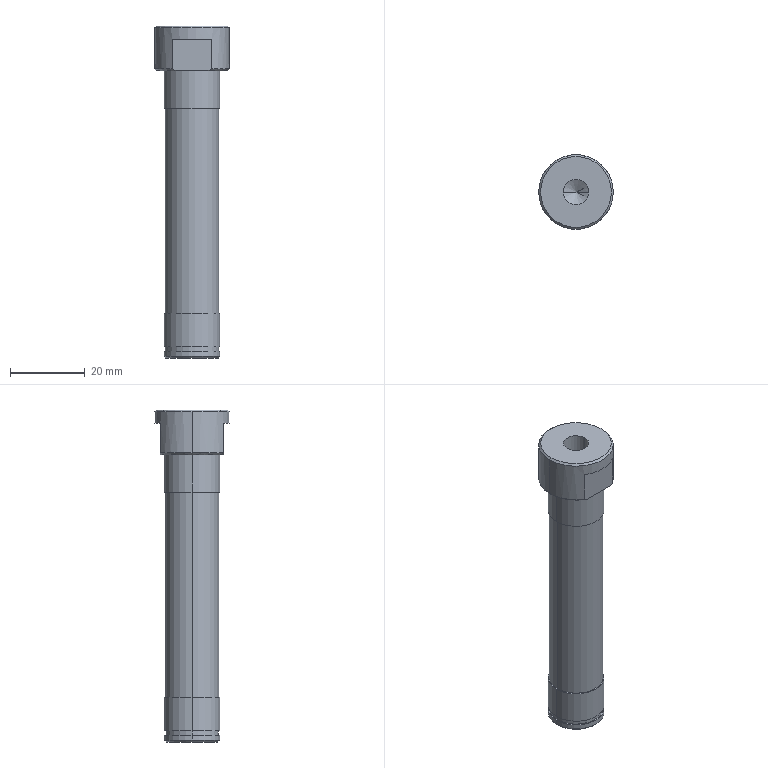Part | STEP file | 10000020461swp000-1 | 1 solid | 34 faces | box 20 x 20 x 89 mm | volume 15653 mm3 | cylinder 14 | plane 11 | cone 9 | commonest cylinder face diameters 15 x6 6.8 x2 14.3 x2 14.4 x2 20 x2
STEP:
#1=CARTESIAN_POINT('',(9.5,0.,0.));
#2=VERTEX_POINT('',#1);
#3=CARTESIAN_POINT('',(-9.5,0.,0.));
#4=VERTEX_POINT('',#3);
#5=CARTESIAN_POINT('',(0.,0.,0.));
#6=DIRECTION('',(0.,0.,1.));
#7=DIRECTION('',(1.,0.,0.));
#8=AXIS2_PLACEMENT_3D('',#5,#6,#7);
#9=CIRCLE('',#8,9.5);
#10=EDGE_CURVE('',#2,#4,#9,.T.);
#11=ORIENTED_EDGE('',*,*,#10,.F.);
#12=CARTESIAN_POINT('',(10.,0.,-0.5));
#13=VERTEX_POINT('',#12);
#14=CARTESIAN_POINT('',(9.5,0.,0.));
#15=DIRECTION('',(0.7071,0.,-0.7071));
#16=VECTOR('',#15,1000.);
#17=LINE('',#14,#16);
#18=EDGE_CURVE('',#2,#13,#17,.T.);
#19=ORIENTED_EDGE('',*,*,#18,.T.);
#20=CARTESIAN_POINT('',(-10.,0.,-0.5));
#21=VERTEX_POINT('',#20);
#22=CARTESIAN_POINT('',(0.,0.,-0.5));
#23=DIRECTION('',(0.,0.,-1.));
#24=DIRECTION('',(1.,0.,0.));
#25=AXIS2_PLACEMENT_3D('',#22,#23,#24);
#26=CIRCLE('',#25,10.);
#27=EDGE_CURVE('',#21,#13,#26,.T.);
#28=ORIENTED_EDGE('',*,*,#27,.F.);
#29=CARTESIAN_POINT('',(-9.5,0.,0.));
#30=DIRECTION('',(-0.7071,0.,-0.7071));
#31=VECTOR('',#30,1000.);
#32=LINE('',#29,#31);
#33=EDGE_CURVE('',#4,#21,#32,.T.);
#34=ORIENTED_EDGE('',*,*,#33,.F.);
#35=EDGE_LOOP('',(#11,#19,#28,#34));
#36=FACE_OUTER_BOUND('',#35,.T.);
#37=CARTESIAN_POINT('',(0.,0.,0.));
#38=DIRECTION('',(0.,0.,-1.));
#39=DIRECTION('',(-1.,0.,0.));
#40=AXIS2_PLACEMENT_3D('',#37,#38,#39);
#41=CONICAL_SURFACE('',#40,9.5,0.7854);
#42=ADVANCED_FACE('',(#36),#41,.T.);
#43=CARTESIAN_POINT('',(-7.,0.,-89.));
#44=VERTEX_POINT('',#43);
#45=CARTESIAN_POINT('',(7.,0.,-89.));
#46=VERTEX_POINT('',#45);
#47=CARTESIAN_POINT('',(0.,0.,-89.));
#48=DIRECTION('',(0.,0.,-1.));
#49=DIRECTION('',(-1.,0.,0.));
#50=AXIS2_PLACEMENT_3D('',#47,#48,#49);
#51=CIRCLE('',#50,7.);
#52=EDGE_CURVE('',#44,#46,#51,.T.);
#53=ORIENTED_EDGE('',*,*,#52,.F.);
#54=CARTESIAN_POINT('',(-7.5,0.,-88.5));
#55=VERTEX_POINT('',#54);
#56=CARTESIAN_POINT('',(-7.,0.,-89.));
#57=DIRECTION('',(-0.7071,0.,0.7071));
#58=VECTOR('',#57,1000.);
#59=LINE('',#56,#58);
#60=EDGE_CURVE('',#44,#55,#59,.T.);
#61=ORIENTED_EDGE('',*,*,#60,.T.);
#62=CARTESIAN_POINT('',(7.5,0.,-88.5));
#63=VERTEX_POINT('',#62);
#64=CARTESIAN_POINT('',(0.,0.,-88.5));
#65=DIRECTION('',(0.,0.,1.));
#66=DIRECTION('',(-1.,0.,0.));
#67=AXIS2_PLACEMENT_3D('',#64,#65,#66);
#68=CIRCLE('',#67,7.5);
#69=EDGE_CURVE('',#63,#55,#68,.T.);
#70=ORIENTED_EDGE('',*,*,#69,.F.);
#71=CARTESIAN_POINT('',(7.,0.,-89.));
#72=DIRECTION('',(0.7071,0.,0.7071));
#73=VECTOR('',#72,1000.);
#74=LINE('',#71,#73);
#75=EDGE_CURVE('',#46,#63,#74,.T.);
#76=ORIENTED_EDGE('',*,*,#75,.F.);
#77=EDGE_LOOP('',(#53,#61,#70,#76));
#78=FACE_OUTER_BOUND('',#77,.T.);
#79=CARTESIAN_POINT('',(0.,0.,-89.));
#80=DIRECTION('',(0.,0.,1.));
#81=DIRECTION('',(1.,0.,0.));
#82=AXIS2_PLACEMENT_3D('',#79,#80,#81);
#83=CONICAL_SURFACE('',#82,7.,0.7854);
#84=ADVANCED_FACE('',(#78),#83,.T.);
#85=CARTESIAN_POINT('',(9.5,0.,-12.));
#86=VERTEX_POINT('',#85);
#87=CARTESIAN_POINT('',(4.243,-8.5,-12.));
#88=VERTEX_POINT('',#87);
#89=CARTESIAN_POINT('',(0.,0.,-12.));
#90=DIRECTION('',(0.,0.,-1.));
#91=DIRECTION('',(1.,0.,0.));
#92=AXIS2_PLACEMENT_3D('',#89,#90,#91);
#93=CIRCLE('',#92,9.5);
#94=EDGE_CURVE('',#86,#88,#93,.T.);
#95=ORIENTED_EDGE('',*,*,#94,.F.);
#96=CARTESIAN_POINT('',(10.,0.,-11.5));
#97=VERTEX_POINT('',#96);
#98=CARTESIAN_POINT('',(10.,0.,-11.5));
#99=DIRECTION('',(0.7071,0.,0.7071));
#100=VECTOR('',#99,1000.);
#101=LINE('',#98,#100);
#102=EDGE_CURVE('',#86,#97,#101,.T.);
#103=ORIENTED_EDGE('',*,*,#102,.T.);
#104=CARTESIAN_POINT('',(5.268,-8.5,-11.5));
#105=VERTEX_POINT('',#104);
#106=CARTESIAN_POINT('',(0.,0.,-11.5));
#107=DIRECTION('',(0.,0.,1.));
#108=DIRECTION('',(1.,0.,0.));
#109=AXIS2_PLACEMENT_3D('',#106,#107,#108);
#110=CIRCLE('',#109,10.);
#111=EDGE_CURVE('',#105,#97,#110,.T.);
#112=ORIENTED_EDGE('',*,*,#111,.F.);
#113=CARTESIAN_POINT('',(4.243,-8.5,-12.));
#114=CARTESIAN_POINT('',(4.59,-8.5,-11.845));
#115=CARTESIAN_POINT('',(4.931,-8.5,-11.677));
#116=CARTESIAN_POINT('',(5.268,-8.5,-11.5));
#117=B_SPLINE_CURVE_WITH_KNOTS('',3,(#113,#114,#115,#116),.UNSPECIFIED.,.F.,.F.,(4,4),(0.,0.001141),.UNSPECIFIED.);
#118=EDGE_CURVE('',#88,#105,#117,.T.);
#119=ORIENTED_EDGE('',*,*,#118,.F.);
#120=EDGE_LOOP('',(#95,#103,#112,#119));
#121=FACE_OUTER_BOUND('',#120,.T.);
#122=CARTESIAN_POINT('',(0.,0.,-11.5));
#123=DIRECTION('',(0.,0.,1.));
#124=DIRECTION('',(1.,0.,0.));
#125=AXIS2_PLACEMENT_3D('',#122,#123,#124);
#126=CONICAL_SURFACE('',#125,10.,0.7854);
#127=ADVANCED_FACE('',(#121),#126,.T.);
#128=CARTESIAN_POINT('',(-3.4,0.,-19.75));
#129=VERTEX_POINT('',#128);
#130=CARTESIAN_POINT('',(3.4,0.,-19.75));
#131=VERTEX_POINT('',#130);
#132=CARTESIAN_POINT('',(0.,0.,-19.75));
#133=DIRECTION('',(0.,0.,1.));
#134=DIRECTION('',(1.,0.,0.));
#135=AXIS2_PLACEMENT_3D('',#132,#133,#134);
#136=CIRCLE('',#135,3.4);
#137=EDGE_CURVE('',#129,#131,#136,.T.);
#138=ORIENTED_EDGE('',*,*,#137,.F.);
#139=CARTESIAN_POINT('',(-3.4,0.,0.));
#140=VERTEX_POINT('',#139);
#141=CARTESIAN_POINT('',(-3.4,0.,0.));
#142=DIRECTION('',(0.,0.,1.));
#143=VECTOR('',#142,1000.);
#144=LINE('',#141,#143);
#145=EDGE_CURVE('',#129,#140,#144,.T.);
#146=ORIENTED_EDGE('',*,*,#145,.T.);
#147=CARTESIAN_POINT('',(3.4,0.,0.));
#148=VERTEX_POINT('',#147);
#149=CARTESIAN_POINT('',(0.,0.,0.));
#150=DIRECTION('',(0.,0.,1.));
#151=DIRECTION('',(1.,0.,0.));
#152=AXIS2_PLACEMENT_3D('',#149,#150,#151);
#153=CIRCLE('',#152,3.4);
#154=EDGE_CURVE('',#140,#148,#153,.T.);
#155=ORIENTED_EDGE('',*,*,#154,.T.);
#156=CARTESIAN_POINT('',(3.4,0.,0.));
#157=DIRECTION('',(0.,0.,1.));
#158=VECTOR('',#157,1000.);
#159=LINE('',#156,#158);
#160=EDGE_CURVE('',#131,#148,#159,.T.);
#161=ORIENTED_EDGE('',*,*,#160,.F.);
#162=EDGE_LOOP('',(#138,#146,#155,#161));
#163=FACE_OUTER_BOUND('',#162,.T.);
#164=CARTESIAN_POINT('',(0.,0.,0.));
#165=DIRECTION('',(0.,0.,1.));
#166=DIRECTION('',(1.,0.,0.));
#167=AXIS2_PLACEMENT_3D('',#164,#165,#166);
#168=CYLINDRICAL_SURFACE('',#167,3.4);
#169=ADVANCED_FACE('',(#163),#168,.F.);
#170=CARTESIAN_POINT('',(0.,0.,-21.793));
#171=VERTEX_POINT('',#170);
#172=CARTESIAN_POINT('',(3.4,0.,-19.75));
#173=DIRECTION('',(0.8572,0.,0.515));
#174=VECTOR('',#173,1000.);
#175=LINE('',#172,#174);
#176=EDGE_CURVE('',#171,#131,#175,.T.);
#177=ORIENTED_EDGE('',*,*,#176,.F.);
#178=CARTESIAN_POINT('',(-3.4,0.,-19.75));
#179=DIRECTION('',(-0.8572,0.,0.515));
#180=VECTOR('',#179,1000.);
#181=LINE('',#178,#180);
#182=EDGE_CURVE('',#171,#129,#181,.T.);
#183=ORIENTED_EDGE('',*,*,#182,.T.);
#184=ORIENTED_EDGE('',*,*,#137,.T.);
#185=EDGE_LOOP('',(#177,#183,#184));
#186=FACE_OUTER_BOUND('',#185,.T.);
#187=CARTESIAN_POINT('',(0.,0.,-19.75));
#188=DIRECTION('',(0.,0.,1.));
#189=DIRECTION('',(1.,0.,0.));
#190=AXIS2_PLACEMENT_3D('',#187,#188,#189);
#191=CONICAL_SURFACE('',#190,3.4,1.03);
#192=ADVANCED_FACE('',(#186),#191,.F.);
#193=ORIENTED_EDGE('',*,*,#69,.T.);
#194=CARTESIAN_POINT('',(-7.5,0.,-87.2));
#195=VERTEX_POINT('',#194);
#196=CARTESIAN_POINT('',(-7.5,0.,-89.));
#197=DIRECTION('',(0.,0.,1.));
#198=VECTOR('',#197,1000.);
#199=LINE('',#196,#198);
#200=EDGE_CURVE('',#55,#195,#199,.T.);
#201=ORIENTED_EDGE('',*,*,#200,.T.);
#202=CARTESIAN_POINT('',(7.5,0.,-87.2));
#203=VERTEX_POINT('',#202);
#204=CARTESIAN_POINT('',(0.,0.,-87.2));
#205=DIRECTION('',(0.,0.,-1.));
#206=DIRECTION('',(-1.,0.,0.));
#207=AXIS2_PLACEMENT_3D('',#204,#205,#206);
#208=CIRCLE('',#207,7.5);
#209=EDGE_CURVE('',#195,#203,#208,.T.);
#210=ORIENTED_EDGE('',*,*,#209,.T.);
#211=CARTESIAN_POINT('',(7.5,0.,-89.));
#212=DIRECTION('',(0.,0.,1.));
#213=VECTOR('',#212,1000.);
#214=LINE('',#211,#213);
#215=EDGE_CURVE('',#63,#203,#214,.T.);
#216=ORIENTED_EDGE('',*,*,#215,.F.);
#217=EDGE_LOOP('',(#193,#201,#210,#216));
#218=FACE_OUTER_BOUND('',#217,.T.);
#219=CARTESIAN_POINT('',(0.,0.,-89.));
#220=DIRECTION('',(0.,0.,1.));
#221=DIRECTION('',(1.,0.,0.));
#222=AXIS2_PLACEMENT_3D('',#219,#220,#221);
#223=CYLINDRICAL_SURFACE('',#222,7.5);
#224=ADVANCED_FACE('',(#218),#223,.T.);
#225=CARTESIAN_POINT('',(-7.15,0.,-86.));
#226=VERTEX_POINT('',#225);
#227=CARTESIAN_POINT('',(7.15,0.,-86.));
#228=VERTEX_POINT('',#227);
#229=CARTESIAN_POINT('',(0.,0.,-86.));
#230=DIRECTION('',(0.,0.,-1.));
#231=DIRECTION('',(-1.,0.,0.));
#232=AXIS2_PLACEMENT_3D('',#229,#230,#231);
#233=CIRCLE('',#232,7.15);
#234=EDGE_CURVE('',#226,#228,#233,.T.);
#235=ORIENTED_EDGE('',*,*,#234,.T.);
#236=CARTESIAN_POINT('',(7.15,0.,-87.2));
#237=VERTEX_POINT('',#236);
#238=CARTESIAN_POINT('',(7.15,0.,-89.));
#239=DIRECTION('',(0.,0.,-1.));
#240=VECTOR('',#239,1000.);
#241=LINE('',#238,#240);
#242=EDGE_CURVE('',#228,#237,#241,.T.);
#243=ORIENTED_EDGE('',*,*,#242,.T.);
#244=CARTESIAN_POINT('',(-7.15,0.,-87.2));
#245=VERTEX_POINT('',#244);
#246=CARTESIAN_POINT('',(0.,0.,-87.2));
#247=DIRECTION('',(0.,0.,-1.));
#248=DIRECTION('',(-1.,0.,0.));
#249=AXIS2_PLACEMENT_3D('',#246,#247,#248);
#250=CIRCLE('',#249,7.15);
#251=EDGE_CURVE('',#245,#237,#250,.T.);
#252=ORIENTED_EDGE('',*,*,#251,.F.);
#253=CARTESIAN_POINT('',(-7.15,0.,-89.));
#254=DIRECTION('',(0.,0.,-1.));
#255=VECTOR('',#254,1000.);
#256=LINE('',#253,#255);
#257=EDGE_CURVE('',#226,#245,#256,.T.);
#258=ORIENTED_EDGE('',*,*,#257,.F.);
#259=EDGE_LOOP('',(#235,#243,#252,#258));
#260=FACE_OUTER_BOUND('',#259,.T.);
#261=CARTESIAN_POINT('',(0.,0.,-89.));
#262=DIRECTION('',(0.,0.,-1.));
#263=DIRECTION('',(-1.,0.,0.));
#264=AXIS2_PLACEMENT_3D('',#261,#262,#263);
#265=CYLINDRICAL_SURFACE('',#264,7.15);
#266=ADVANCED_FACE('',(#260),#265,.T.);
#267=CARTESIAN_POINT('',(-7.2,0.,-77.));
#268=VERTEX_POINT('',#267);
#269=CARTESIAN_POINT('',(7.2,0.,-77.));
#270=VERTEX_POINT('',#269);
#271=CARTESIAN_POINT('',(0.,0.,-77.));
#272=DIRECTION('',(0.,0.,-1.));
#273=DIRECTION('',(-1.,0.,0.));
#274=AXIS2_PLACEMENT_3D('',#271,#272,#273);
#275=CIRCLE('',#274,7.2);
#276=EDGE_CURVE('',#268,#270,#275,.T.);
#277=ORIENTED_EDGE('',*,*,#276,.F.);
#278=CARTESIAN_POINT('',(-7.2,0.,-22.));
#279=VERTEX_POINT('',#278);
#280=CARTESIAN_POINT('',(-7.2,0.,-77.));
#281=DIRECTION('',(0.,0.,1.));
#282=VECTOR('',#281,1000.);
#283=LINE('',#280,#282);
#284=EDGE_CURVE('',#268,#279,#283,.T.);
#285=ORIENTED_EDGE('',*,*,#284,.T.);
#286=CARTESIAN_POINT('',(7.2,0.,-22.));
#287=VERTEX_POINT('',#286);
#288=CARTESIAN_POINT('',(0.,0.,-22.));
#289=DIRECTION('',(0.,0.,-1.));
#290=DIRECTION('',(-1.,0.,0.));
#291=AXIS2_PLACEMENT_3D('',#288,#289,#290);
#292=CIRCLE('',#291,7.2);
#293=EDGE_CURVE('',#279,#287,#292,.T.);
#294=ORIENTED_EDGE('',*,*,#293,.T.);
#295=CARTESIAN_POINT('',(7.2,0.,-77.));
#296=DIRECTION('',(0.,0.,1.));
#297=VECTOR('',#296,1000.);
#298=LINE('',#295,#297);
#299=EDGE_CURVE('',#270,#287,#298,.T.);
#300=ORIENTED_EDGE('',*,*,#299,.F.);
#301=EDGE_LOOP('',(#277,#285,#294,#300));
#302=FACE_OUTER_BOUND('',#301,.T.);
#303=CARTESIAN_POINT('',(0.,0.,-77.));
#304=DIRECTION('',(0.,0.,1.));
#305=DIRECTION('',(1.,0.,0.));
#306=AXIS2_PLACEMENT_3D('',#303,#304,#305);
#307=CYLINDRICAL_SURFACE('',#306,7.2);
#308=ADVANCED_FACE('',(#302),#307,.T.);
#309=CARTESIAN_POINT('',(-7.5,0.,-22.));
#310=VERTEX_POINT('',#309);
#311=CARTESIAN_POINT('',(7.5,0.,-22.));
#312=VERTEX_POINT('',#311);
#313=CARTESIAN_POINT('',(0.,0.,-22.));
#314=DIRECTION('',(0.,0.,-1.));
#315=DIRECTION('',(-1.,0.,0.));
#316=AXIS2_PLACEMENT_3D('',#313,#314,#315);
#317=CIRCLE('',#316,7.5);
#318=EDGE_CURVE('',#310,#312,#317,.T.);
#319=ORIENTED_EDGE('',*,*,#318,.F.);
#320=CARTESIAN_POINT('',(-7.5,0.,-12.));
#321=VERTEX_POINT('',#320);
#322=CARTESIAN_POINT('',(-7.5,0.,-22.));
#323=DIRECTION('',(0.,0.,1.));
#324=VECTOR('',#323,1000.);
#325=LINE('',#322,#324);
#326=EDGE_CURVE('',#310,#321,#325,.T.);
#327=ORIENTED_EDGE('',*,*,#326,.T.);
#328=CARTESIAN_POINT('',(7.5,0.,-12.));
#329=VERTEX_POINT('',#328);
#330=CARTESIAN_POINT('',(0.,0.,-12.));
#331=DIRECTION('',(0.,0.,-1.));
#332=DIRECTION('',(1.,0.,0.));
#333=AXIS2_PLACEMENT_3D('',#330,#331,#332);
#334=CIRCLE('',#333,7.5);
#335=EDGE_CURVE('',#321,#329,#334,.T.);
#336=ORIENTED_EDGE('',*,*,#335,.T.);
#337=CARTESIAN_POINT('',(7.5,0.,-22.));
#338=DIRECTION('',(0.,0.,1.));
#339=VECTOR('',#338,1000.);
#340=LINE('',#337,#339);
#341=EDGE_CURVE('',#312,#329,#340,.T.);
#342=ORIENTED_EDGE('',*,*,#341,.F.);
#343=EDGE_LOOP('',(#319,#327,#336,#342));
#344=FACE_OUTER_BOUND('',#343,.T.);
#345=CARTESIAN_POINT('',(0.,0.,-22.));
#346=DIRECTION('',(0.,0.,1.));
#347=DIRECTION('',(1.,0.,0.));
#348=AXIS2_PLACEMENT_3D('',#345,#346,#347);
#349=CYLINDRICAL_SURFACE('',#348,7.5);
#350=ADVANCED_FACE('',(#344),#349,.T.);
#351=CARTESIAN_POINT('',(-7.5,0.,-86.));
#352=VERTEX_POINT('',#351);
#353=CARTESIAN_POINT('',(7.5,0.,-86.));
#354=VERTEX_POINT('',#353);
#355=CARTESIAN_POINT('',(0.,0.,-86.));
#356=DIRECTION('',(0.,0.,-1.));
#357=DIRECTION('',(-1.,0.,0.));
#358=AXIS2_PLACEMENT_3D('',#355,#356,#357);
#359=CIRCLE('',#358,7.5);
#360=EDGE_CURVE('',#352,#354,#359,.T.);
#361=ORIENTED_EDGE('',*,*,#360,.F.);
#362=CARTESIAN_POINT('',(-7.5,0.,-77.));
#363=VERTEX_POINT('',#362);
#364=CARTESIAN_POINT('',(-7.5,0.,-89.));
#365=DIRECTION('',(0.,0.,1.));
#366=VECTOR('',#365,1000.);
#367=LINE('',#364,#366);
#368=EDGE_CURVE('',#352,#363,#367,.T.);
#369=ORIENTED_EDGE('',*,*,#368,.T.);
#370=CARTESIAN_POINT('',(7.5,0.,-77.));
#371=VERTEX_POINT('',#370);
#372=CARTESIAN_POINT('',(0.,0.,-77.));
#373=DIRECTION('',(0.,0.,-1.));
#374=DIRECTION('',(-1.,0.,0.));
#375=AXIS2_PLACEMENT_3D('',#372,#373,#374);
#376=CIRCLE('',#375,7.5);
#377=EDGE_CURVE('',#363,#371,#376,.T.);
#378=ORIENTED_EDGE('',*,*,#377,.T.);
#379=CARTESIAN_POINT('',(7.5,0.,-89.));
#380=DIRECTION('',(0.,0.,1.));
#381=VECTOR('',#380,1000.);
#382=LINE('',#379,#381);
#383=EDGE_CURVE('',#354,#371,#382,.T.);
#384=ORIENTED_EDGE('',*,*,#383,.F.);
#385=EDGE_LOOP('',(#361,#369,#378,#384));
#386=FACE_OUTER_BOUND('',#385,.T.);
#387=CARTESIAN_POINT('',(0.,0.,-89.));
#388=DIRECTION('',(0.,0.,1.));
#389=DIRECTION('',(1.,0.,0.));
#390=AXIS2_PLACEMENT_3D('',#387,#388,#389);
#391=CYLINDRICAL_SURFACE('',#390,7.5);
#392=ADVANCED_FACE('',(#386),#391,.T.);
#393=CARTESIAN_POINT('',(-5.268,8.5,-11.5));
#394=VERTEX_POINT('',#393);
#395=CARTESIAN_POINT('',(-10.,0.,-11.5));
#396=VERTEX_POINT('',#395);
#397=CARTESIAN_POINT('',(0.,0.,-11.5));
#398=DIRECTION('',(0.,0.,1.));
#399=DIRECTION('',(1.,0.,0.));
#400=AXIS2_PLACEMENT_3D('',#397,#398,#399);
#401=CIRCLE('',#400,10.);
#402=EDGE_CURVE('',#394,#396,#401,.T.);
#403=ORIENTED_EDGE('',*,*,#402,.T.);
#404=CARTESIAN_POINT('',(-10.,0.,-12.));
#405=DIRECTION('',(0.,0.,1.));
#406=VECTOR('',#405,1000.);
#407=LINE('',#404,#406);
#408=EDGE_CURVE('',#396,#21,#407,.T.);
#409=ORIENTED_EDGE('',*,*,#408,.T.);
#410=ORIENTED_EDGE('',*,*,#27,.T.);
#411=CARTESIAN_POINT('',(10.,0.,-12.));
#412=DIRECTION('',(0.,0.,1.));
#413=VECTOR('',#412,1000.);
#414=LINE('',#411,#413);
#415=EDGE_CURVE('',#97,#13,#414,.T.);
#416=ORIENTED_EDGE('',*,*,#415,.F.);
#417=CARTESIAN_POINT('',(5.268,8.5,-11.5));
#418=VERTEX_POINT('',#417);
#419=CARTESIAN_POINT('',(0.,0.,-11.5));
#420=DIRECTION('',(0.,0.,1.));
#421=DIRECTION('',(1.,0.,0.));
#422=AXIS2_PLACEMENT_3D('',#419,#420,#421);
#423=CIRCLE('',#422,10.);
#424=EDGE_CURVE('',#97,#418,#423,.T.);
#425=ORIENTED_EDGE('',*,*,#424,.T.);
#426=CARTESIAN_POINT('',(5.268,8.5,-3.5));
#427=VERTEX_POINT('',#426);
#428=CARTESIAN_POINT('',(5.268,8.5,-12.));
#429=DIRECTION('',(0.,0.,1.));
#430=VECTOR('',#429,1000.);
#431=LINE('',#428,#430);
#432=EDGE_CURVE('',#418,#427,#431,.T.);
#433=ORIENTED_EDGE('',*,*,#432,.T.);
#434=CARTESIAN_POINT('',(-5.268,8.5,-3.5));
#435=VERTEX_POINT('',#434);
#436=CARTESIAN_POINT('',(0.,0.,-3.5));
#437=DIRECTION('',(0.,0.,1.));
#438=DIRECTION('',(-1.,0.,0.));
#439=AXIS2_PLACEMENT_3D('',#436,#437,#438);
#440=CIRCLE('',#439,10.);
#441=EDGE_CURVE('',#427,#435,#440,.T.);
#442=ORIENTED_EDGE('',*,*,#441,.T.);
#443=CARTESIAN_POINT('',(-5.268,8.5,-12.));
#444=DIRECTION('',(0.,0.,-1.));
#445=VECTOR('',#444,1000.);
#446=LINE('',#443,#445);
#447=EDGE_CURVE('',#435,#394,#446,.T.);
#448=ORIENTED_EDGE('',*,*,#447,.T.);
#449=EDGE_LOOP('',(#403,#409,#410,#416,#425,#433,#442,#448));
#450=FACE_OUTER_BOUND('',#449,.T.);
#451=CARTESIAN_POINT('',(0.,0.,-12.));
#452=DIRECTION('',(0.,0.,1.));
#453=DIRECTION('',(1.,0.,0.));
#454=AXIS2_PLACEMENT_3D('',#451,#452,#453);
#455=CYLINDRICAL_SURFACE('',#454,10.);
#456=ADVANCED_FACE('',(#450),#455,.T.);
#457=ORIENTED_EDGE('',*,*,#408,.F.);
#458=CARTESIAN_POINT('',(-5.268,-8.5,-11.5));
#459=VERTEX_POINT('',#458);
#460=CARTESIAN_POINT('',(0.,0.,-11.5));
#461=DIRECTION('',(0.,0.,1.));
#462=DIRECTION('',(1.,0.,0.));
#463=AXIS2_PLACEMENT_3D('',#460,#461,#462);
#464=CIRCLE('',#463,10.);
#465=EDGE_CURVE('',#396,#459,#464,.T.);
#466=ORIENTED_EDGE('',*,*,#465,.T.);
#467=CARTESIAN_POINT('',(-5.268,-8.5,-3.5));
#468=VERTEX_POINT('',#467);
#469=CARTESIAN_POINT('',(-5.268,-8.5,-12.));
#470=DIRECTION('',(0.,0.,1.));
#471=VECTOR('',#470,1000.);
#472=LINE('',#469,#471);
#473=EDGE_CURVE('',#459,#468,#472,.T.);
#474=ORIENTED_EDGE('',*,*,#473,.T.);
#475=CARTESIAN_POINT('',(5.268,-8.5,-3.5));
#476=VERTEX_POINT('',#475);
#477=CARTESIAN_POINT('',(0.,0.,-3.5));
#478=DIRECTION('',(0.,0.,-1.));
#479=DIRECTION('',(1.,0.,0.));
#480=AXIS2_PLACEMENT_3D('',#477,#478,#479);
#481=CIRCLE('',#480,10.);
#482=EDGE_CURVE('',#476,#468,#481,.T.);
#483=ORIENTED_EDGE('',*,*,#482,.F.);
#484=CARTESIAN_POINT('',(5.268,-8.5,-12.));
#485=DIRECTION('',(0.,0.,-1.));
#486=VECTOR('',#485,1000.);
#487=LINE('',#484,#486);
#488=EDGE_CURVE('',#476,#105,#487,.T.);
#489=ORIENTED_EDGE('',*,*,#488,.T.);
#490=ORIENTED_EDGE('',*,*,#111,.T.);
#491=ORIENTED_EDGE('',*,*,#415,.T.);
#492=CARTESIAN_POINT('',(0.,0.,-0.5));
#493=DIRECTION('',(0.,0.,-1.));
#494=DIRECTION('',(1.,0.,0.));
#495=AXIS2_PLACEMENT_3D('',#492,#493,#494);
#496=CIRCLE('',#495,10.);
#497=EDGE_CURVE('',#13,#21,#496,.T.);
#498=ORIENTED_EDGE('',*,*,#497,.T.);
#499=EDGE_LOOP('',(#457,#466,#474,#483,#489,#490,#491,#498));
#500=FACE_OUTER_BOUND('',#499,.T.);
#501=CARTESIAN_POINT('',(0.,0.,-12.));
#502=DIRECTION('',(0.,0.,1.));
#503=DIRECTION('',(1.,0.,0.));
#504=AXIS2_PLACEMENT_3D('',#501,#502,#503);
#505=CYLINDRICAL_SURFACE('',#504,10.);
#506=ADVANCED_FACE('',(#500),#505,.T.);
#507=CARTESIAN_POINT('',(0.,0.,-12.));
#508=DIRECTION('',(0.,0.,-1.));
#509=DIRECTION('',(1.,0.,0.));
#510=AXIS2_PLACEMENT_3D('',#507,#508,#509);
#511=CIRCLE('',#510,7.5);
#512=EDGE_CURVE('',#329,#321,#511,.T.);
#513=ORIENTED_EDGE('',*,*,#512,.F.);
#514=ORIENTED_EDGE('',*,*,#335,.F.);
#515=EDGE_LOOP('',(#513,#514));
#516=FACE_BOUND('',#515,.T.);
#517=CARTESIAN_POINT('',(4.243,8.5,-12.));
#518=VERTEX_POINT('',#517);
#519=CARTESIAN_POINT('',(-4.243,8.5,-12.));
#520=VERTEX_POINT('',#519);
#521=CARTESIAN_POINT('',(0.,8.5,-12.));
#522=DIRECTION('',(-1.,0.,0.));
#523=VECTOR('',#522,1000.);
#524=LINE('',#521,#523);
#525=EDGE_CURVE('',#518,#520,#524,.T.);
#526=ORIENTED_EDGE('',*,*,#525,.F.);
#527=CARTESIAN_POINT('',(0.,0.,-12.));
#528=DIRECTION('',(0.,0.,-1.));
#529=DIRECTION('',(1.,0.,0.));
#530=AXIS2_PLACEMENT_3D('',#527,#528,#529);
#531=CIRCLE('',#530,9.5);
#532=EDGE_CURVE('',#518,#86,#531,.T.);
#533=ORIENTED_EDGE('',*,*,#532,.T.);
#534=ORIENTED_EDGE('',*,*,#94,.T.);
#535=CARTESIAN_POINT('',(-4.243,-8.5,-12.));
#536=VERTEX_POINT('',#535);
#537=CARTESIAN_POINT('',(0.,-8.5,-12.));
#538=DIRECTION('',(1.,0.,0.));
#539=VECTOR('',#538,1000.);
#540=LINE('',#537,#539);
#541=EDGE_CURVE('',#536,#88,#540,.T.);
#542=ORIENTED_EDGE('',*,*,#541,.F.);
#543=CARTESIAN_POINT('',(0.,0.,-12.));
#544=DIRECTION('',(0.,0.,-1.));
#545=DIRECTION('',(1.,0.,0.));
#546=AXIS2_PLACEMENT_3D('',#543,#544,#545);
#547=CIRCLE('',#546,9.5);
#548=EDGE_CURVE('',#536,#520,#547,.T.);
#549=ORIENTED_EDGE('',*,*,#548,.T.);
#550=EDGE_LOOP('',(#526,#533,#534,#542,#549));
#551=FACE_OUTER_BOUND('',#550,.T.);
#552=CARTESIAN_POINT('',(0.,0.,-12.));
#553=DIRECTION('',(0.,0.,1.));
#554=DIRECTION('',(1.,0.,0.));
#555=AXIS2_PLACEMENT_3D('',#552,#553,#554);
#556=PLANE('',#555);
#557=ADVANCED_FACE('',(#516,#551),#556,.F.);
#558=ORIENTED_EDGE('',*,*,#368,.F.);
#559=CARTESIAN_POINT('',(0.,0.,-86.));
#560=DIRECTION('',(0.,0.,-1.));
#561=DIRECTION('',(-1.,0.,0.));
#562=AXIS2_PLACEMENT_3D('',#559,#560,#561);
#563=CIRCLE('',#562,7.5);
#564=EDGE_CURVE('',#354,#352,#563,.T.);
#565=ORIENTED_EDGE('',*,*,#564,.F.);
#566=ORIENTED_EDGE('',*,*,#383,.T.);
#567=CARTESIAN_POINT('',(0.,0.,-77.));
#568=DIRECTION('',(0.,0.,-1.));
#569=DIRECTION('',(-1.,0.,0.));
#570=AXIS2_PLACEMENT_3D('',#567,#568,#569);
#571=CIRCLE('',#570,7.5);
#572=EDGE_CURVE('',#371,#363,#571,.T.);
#573=ORIENTED_EDGE('',*,*,#572,.T.);
#574=EDGE_LOOP('',(#558,#565,#566,#573));
#575=FACE_OUTER_BOUND('',#574,.T.);
#576=CARTESIAN_POINT('',(0.,0.,-89.));
#577=DIRECTION('',(0.,0.,1.));
#578=DIRECTION('',(1.,0.,0.));
#579=AXIS2_PLACEMENT_3D('',#576,#577,#578);
#580=CYLINDRICAL_SURFACE('',#579,7.5);
#581=ADVANCED_FACE('',(#575),#580,.T.);
#582=CARTESIAN_POINT('',(0.,0.,0.));
#583=DIRECTION('',(0.,0.,1.));
#584=DIRECTION('',(1.,0.,0.));
#585=AXIS2_PLACEMENT_3D('',#582,#583,#584);
#586=CIRCLE('',#585,9.5);
#587=EDGE_CURVE('',#4,#2,#586,.T.);
#588=ORIENTED_EDGE('',*,*,#587,.T.);
#589=ORIENTED_EDGE('',*,*,#10,.T.);
#590=EDGE_LOOP('',(#588,#589));
#591=FACE_OUTER_BOUND('',#590,.T.);
#592=CARTESIAN_POINT('',(0.,0.,0.));
#593=DIRECTION('',(0.,0.,1.));
#594=DIRECTION('',(1.,0.,0.));
#595=AXIS2_PLACEMENT_3D('',#592,#593,#594);
#596=CIRCLE('',#595,3.4);
#597=EDGE_CURVE('',#148,#140,#596,.T.);
#598=ORIENTED_EDGE('',*,*,#597,.F.);
#599=ORIENTED_EDGE('',*,*,#154,.F.);
#600=EDGE_LOOP('',(#598,#599));
#601=FACE_BOUND('',#600,.T.);
#602=CARTESIAN_POINT('',(0.,0.,0.));
#603=DIRECTION('',(0.,0.,1.));
#604=DIRECTION('',(1.,0.,0.));
#605=AXIS2_PLACEMENT_3D('',#602,#603,#604);
#606=PLANE('',#605);
#607=ADVANCED_FACE('',(#591,#601),#606,.T.);
#608=ORIENTED_EDGE('',*,*,#326,.F.);
#609=CARTESIAN_POINT('',(0.,0.,-22.));
#610=DIRECTION('',(0.,0.,-1.));
#611=DIRECTION('',(-1.,0.,0.));
#612=AXIS2_PLACEMENT_3D('',#609,#610,#611);
#613=CIRCLE('',#612,7.5);
#614=EDGE_CURVE('',#312,#310,#613,.T.);
#615=ORIENTED_EDGE('',*,*,#614,.F.);
#616=ORIENTED_EDGE('',*,*,#341,.T.);
#617=ORIENTED_EDGE('',*,*,#512,.T.);
#618=EDGE_LOOP('',(#608,#615,#616,#617));
#619=FACE_OUTER_BOUND('',#618,.T.);
#620=CARTESIAN_POINT('',(0.,0.,-22.));
#621=DIRECTION('',(0.,0.,1.));
#622=DIRECTION('',(1.,0.,0.));
#623=AXIS2_PLACEMENT_3D('',#620,#621,#622);
#624=CYLINDRICAL_SURFACE('',#623,7.5);
#625=ADVANCED_FACE('',(#619),#624,.T.);
#626=CARTESIAN_POINT('',(0.,0.,-22.));
#627=DIRECTION('',(0.,0.,-1.));
#628=DIRECTION('',(-1.,0.,0.));
#629=AXIS2_PLACEMENT_3D('',#626,#627,#628);
#630=CIRCLE('',#629,7.2);
#631=EDGE_CURVE('',#287,#279,#630,.T.);
#632=ORIENTED_EDGE('',*,*,#631,.F.);
#633=ORIENTED_EDGE('',*,*,#293,.F.);
#634=EDGE_LOOP('',(#632,#633));
#635=FACE_BOUND('',#634,.T.);
#636=ORIENTED_EDGE('',*,*,#614,.T.);
#637=ORIENTED_EDGE('',*,*,#318,.T.);
#638=EDGE_LOOP('',(#636,#637));
#639=FACE_OUTER_BOUND('',#638,.T.);
#640=CARTESIAN_POINT('',(0.,0.,-22.));
#641=DIRECTION('',(0.,0.,-1.));
#642=DIRECTION('',(-1.,0.,0.));
#643=AXIS2_PLACEMENT_3D('',#640,#641,#642);
#644=PLANE('',#643);
#645=ADVANCED_FACE('',(#635,#639),#644,.T.);
#646=ORIENTED_EDGE('',*,*,#284,.F.);
#647=CARTESIAN_POINT('',(0.,0.,-77.));
#648=DIRECTION('',(0.,0.,-1.));
#649=DIRECTION('',(-1.,0.,0.));
#650=AXIS2_PLACEMENT_3D('',#647,#648,#649);
#651=CIRCLE('',#650,7.2);
#652=EDGE_CURVE('',#270,#268,#651,.T.);
#653=ORIENTED_EDGE('',*,*,#652,.F.);
#654=ORIENTED_EDGE('',*,*,#299,.T.);
#655=ORIENTED_EDGE('',*,*,#631,.T.);
#656=EDGE_LOOP('',(#646,#653,#654,#655));
#657=FACE_OUTER_BOUND('',#656,.T.);
#658=CARTESIAN_POINT('',(0.,0.,-77.));
#659=DIRECTION('',(0.,0.,1.));
#660=DIRECTION('',(1.,0.,0.));
#661=AXIS2_PLACEMENT_3D('',#658,#659,#660);
#662=CYLINDRICAL_SURFACE('',#661,7.2);
#663=ADVANCED_FACE('',(#657),#662,.T.);
#664=ORIENTED_EDGE('',*,*,#652,.T.);
#665=ORIENTED_EDGE('',*,*,#276,.T.);
#666=EDGE_LOOP('',(#664,#665));
#667=FACE_BOUND('',#666,.T.);
#668=ORIENTED_EDGE('',*,*,#572,.F.);
#669=ORIENTED_EDGE('',*,*,#377,.F.);
#670=EDGE_LOOP('',(#668,#669));
#671=FACE_OUTER_BOUND('',#670,.T.);
#672=CARTESIAN_POINT('',(0.,0.,-77.));
#673=DIRECTION('',(0.,0.,-1.));
#674=DIRECTION('',(-1.,0.,0.));
#675=AXIS2_PLACEMENT_3D('',#672,#673,#674);
#676=PLANE('',#675);
#677=ADVANCED_FACE('',(#667,#671),#676,.F.);
#678=ORIENTED_EDGE('',*,*,#242,.F.);
#679=CARTESIAN_POINT('',(0.,0.,-86.));
#680=DIRECTION('',(0.,0.,-1.));
#681=DIRECTION('',(-1.,0.,0.));
#682=AXIS2_PLACEMENT_3D('',#679,#680,#681);
#683=CIRCLE('',#682,7.15);
#684=EDGE_CURVE('',#228,#226,#683,.T.);
#685=ORIENTED_EDGE('',*,*,#684,.T.);
#686=ORIENTED_EDGE('',*,*,#257,.T.);
#687=CARTESIAN_POINT('',(0.,0.,-87.2));
#688=DIRECTION('',(0.,0.,-1.));
#689=DIRECTION('',(-1.,0.,0.));
#690=AXIS2_PLACEMENT_3D('',#687,#688,#689);
#691=CIRCLE('',#690,7.15);
#692=EDGE_CURVE('',#237,#245,#691,.T.);
#693=ORIENTED_EDGE('',*,*,#692,.F.);
#694=EDGE_LOOP('',(#678,#685,#686,#693));
#695=FACE_OUTER_BOUND('',#694,.T.);
#696=CARTESIAN_POINT('',(0.,0.,-89.));
#697=DIRECTION('',(0.,0.,-1.));
#698=DIRECTION('',(-1.,0.,0.));
#699=AXIS2_PLACEMENT_3D('',#696,#697,#698);
#700=CYLINDRICAL_SURFACE('',#699,7.15);
#701=ADVANCED_FACE('',(#695),#700,.T.);
#702=ORIENTED_EDGE('',*,*,#564,.T.);
#703=ORIENTED_EDGE('',*,*,#360,.T.);
#704=EDGE_LOOP('',(#702,#703));
#705=FACE_OUTER_BOUND('',#704,.T.);
#706=ORIENTED_EDGE('',*,*,#234,.F.);
#707=ORIENTED_EDGE('',*,*,#684,.F.);
#708=EDGE_LOOP('',(#706,#707));
#709=FACE_BOUND('',#708,.T.);
#710=CARTESIAN_POINT('',(7.15,0.,-86.));
#711=DIRECTION('',(0.,0.,-1.));
#712=DIRECTION('',(-1.,0.,0.));
#713=AXIS2_PLACEMENT_3D('',#710,#711,#712);
#714=PLANE('',#713);
#715=ADVANCED_FACE('',(#705,#709),#714,.T.);
#716=ORIENTED_EDGE('',*,*,#251,.T.);
#717=ORIENTED_EDGE('',*,*,#692,.T.);
#718=EDGE_LOOP('',(#716,#717));
#719=FACE_BOUND('',#718,.T.);
#720=CARTESIAN_POINT('',(0.,0.,-87.2));
#721=DIRECTION('',(0.,0.,-1.));
#722=DIRECTION('',(-1.,0.,0.));
#723=AXIS2_PLACEMENT_3D('',#720,#721,#722);
#724=CIRCLE('',#723,7.5);
#725=EDGE_CURVE('',#203,#195,#724,.T.);
#726=ORIENTED_EDGE('',*,*,#725,.F.);
#727=ORIENTED_EDGE('',*,*,#209,.F.);
#728=EDGE_LOOP('',(#726,#727));
#729=FACE_OUTER_BOUND('',#728,.T.);
#730=CARTESIAN_POINT('',(7.15,0.,-87.2));
#731=DIRECTION('',(0.,0.,1.));
#732=DIRECTION('',(1.,0.,0.));
#733=AXIS2_PLACEMENT_3D('',#730,#731,#732);
#734=PLANE('',#733);
#735=ADVANCED_FACE('',(#719,#729),#734,.T.);
#736=CARTESIAN_POINT('',(0.,0.,-89.));
#737=DIRECTION('',(0.,0.,-1.));
#738=DIRECTION('',(-1.,0.,0.));
#739=AXIS2_PLACEMENT_3D('',#736,#737,#738);
#740=CIRCLE('',#739,7.);
#741=EDGE_CURVE('',#46,#44,#740,.T.);
#742=ORIENTED_EDGE('',*,*,#741,.T.);
#743=ORIENTED_EDGE('',*,*,#52,.T.);
#744=EDGE_LOOP('',(#742,#743));
#745=FACE_OUTER_BOUND('',#744,.T.);
#746=CARTESIAN_POINT('',(0.,0.,-89.));
#747=DIRECTION('',(0.,0.,-1.));
#748=DIRECTION('',(-1.,0.,0.));
#749=AXIS2_PLACEMENT_3D('',#746,#747,#748);
#750=PLANE('',#749);
#751=ADVANCED_FACE('',(#745),#750,.T.);
#752=ORIENTED_EDGE('',*,*,#200,.F.);
#753=CARTESIAN_POINT('',(0.,0.,-88.5));
#754=DIRECTION('',(0.,0.,1.));
#755=DIRECTION('',(-1.,0.,0.));
#756=AXIS2_PLACEMENT_3D('',#753,#754,#755);
#757=CIRCLE('',#756,7.5);
#758=EDGE_CURVE('',#55,#63,#757,.T.);
#759=ORIENTED_EDGE('',*,*,#758,.T.);
#760=ORIENTED_EDGE('',*,*,#215,.T.);
#761=ORIENTED_EDGE('',*,*,#725,.T.);
#762=EDGE_LOOP('',(#752,#759,#760,#761));
#763=FACE_OUTER_BOUND('',#762,.T.);
#764=CARTESIAN_POINT('',(0.,0.,-89.));
#765=DIRECTION('',(0.,0.,1.));
#766=DIRECTION('',(1.,0.,0.));
#767=AXIS2_PLACEMENT_3D('',#764,#765,#766);
#768=CYLINDRICAL_SURFACE('',#767,7.5);
#769=ADVANCED_FACE('',(#763),#768,.T.);
#770=ORIENTED_EDGE('',*,*,#182,.F.);
#771=ORIENTED_EDGE('',*,*,#176,.T.);
#772=CARTESIAN_POINT('',(0.,0.,-19.75));
#773=DIRECTION('',(0.,0.,1.));
#774=DIRECTION('',(1.,0.,0.));
#775=AXIS2_PLACEMENT_3D('',#772,#773,#774);
#776=CIRCLE('',#775,3.4);
#777=EDGE_CURVE('',#131,#129,#776,.T.);
#778=ORIENTED_EDGE('',*,*,#777,.T.);
#779=EDGE_LOOP('',(#770,#771,#778));
#780=FACE_OUTER_BOUND('',#779,.T.);
#781=CARTESIAN_POINT('',(0.,0.,-19.75));
#782=DIRECTION('',(0.,0.,1.));
#783=DIRECTION('',(1.,0.,0.));
#784=AXIS2_PLACEMENT_3D('',#781,#782,#783);
#785=CONICAL_SURFACE('',#784,3.4,1.03);
#786=ADVANCED_FACE('',(#780),#785,.F.);
#787=ORIENTED_EDGE('',*,*,#145,.F.);
#788=ORIENTED_EDGE('',*,*,#777,.F.);
#789=ORIENTED_EDGE('',*,*,#160,.T.);
#790=ORIENTED_EDGE('',*,*,#597,.T.);
#791=EDGE_LOOP('',(#787,#788,#789,#790));
#792=FACE_OUTER_BOUND('',#791,.T.);
#793=CARTESIAN_POINT('',(0.,0.,0.));
#794=DIRECTION('',(0.,0.,1.));
#795=DIRECTION('',(1.,0.,0.));
#796=AXIS2_PLACEMENT_3D('',#793,#794,#795);
#797=CYLINDRICAL_SURFACE('',#796,3.4);
#798=ADVANCED_FACE('',(#792),#797,.F.);
#799=CARTESIAN_POINT('',(-10.,8.5,-3.5));
#800=DIRECTION('',(1.,0.,0.));
#801=VECTOR('',#800,1000.);
#802=LINE('',#799,#801);
#803=EDGE_CURVE('',#435,#427,#802,.T.);
#804=ORIENTED_EDGE('',*,*,#803,.F.);
#805=ORIENTED_EDGE('',*,*,#441,.F.);
#806=EDGE_LOOP('',(#804,#805));
#807=FACE_OUTER_BOUND('',#806,.T.);
#808=CARTESIAN_POINT('',(-10.,10.,-3.5));
#809=DIRECTION('',(0.,0.,-1.));
#810=DIRECTION('',(-1.,0.,0.));
#811=AXIS2_PLACEMENT_3D('',#808,#809,#810);
#812=PLANE('',#811);
#813=ADVANCED_FACE('',(#807),#812,.T.);
#814=ORIENTED_EDGE('',*,*,#432,.F.);
#815=CARTESIAN_POINT('',(5.268,8.5,-11.5));
#816=CARTESIAN_POINT('',(4.931,8.5,-11.677));
#817=CARTESIAN_POINT('',(4.59,8.5,-11.845));
#818=CARTESIAN_POINT('',(4.243,8.5,-12.));
#819=B_SPLINE_CURVE_WITH_KNOTS('',3,(#815,#816,#817,#818),.UNSPECIFIED.,.F.,.F.,(4,4),(0.,0.001141),.UNSPECIFIED.);
#820=EDGE_CURVE('',#418,#518,#819,.T.);
#821=ORIENTED_EDGE('',*,*,#820,.T.);
#822=ORIENTED_EDGE('',*,*,#525,.T.);
#823=CARTESIAN_POINT('',(-4.243,8.5,-12.));
#824=CARTESIAN_POINT('',(-4.59,8.5,-11.845));
#825=CARTESIAN_POINT('',(-4.931,8.5,-11.677));
#826=CARTESIAN_POINT('',(-5.268,8.5,-11.5));
#827=B_SPLINE_CURVE_WITH_KNOTS('',3,(#823,#824,#825,#826),.UNSPECIFIED.,.F.,.F.,(4,4),(0.,0.001141),.UNSPECIFIED.);
#828=EDGE_CURVE('',#520,#394,#827,.T.);
#829=ORIENTED_EDGE('',*,*,#828,.T.);
#830=ORIENTED_EDGE('',*,*,#447,.F.);
#831=ORIENTED_EDGE('',*,*,#803,.T.);
#832=EDGE_LOOP('',(#814,#821,#822,#829,#830,#831));
#833=FACE_OUTER_BOUND('',#832,.T.);
#834=CARTESIAN_POINT('',(0.,8.5,0.));
#835=DIRECTION('',(0.,1.,0.));
#836=DIRECTION('',(0.,0.,1.));
#837=AXIS2_PLACEMENT_3D('',#834,#835,#836);
#838=PLANE('',#837);
#839=ADVANCED_FACE('',(#833),#838,.T.);
#840=CARTESIAN_POINT('',(-10.,-8.5,-3.5));
#841=DIRECTION('',(1.,0.,0.));
#842=VECTOR('',#841,1000.);
#843=LINE('',#840,#842);
#844=EDGE_CURVE('',#468,#476,#843,.T.);
#845=ORIENTED_EDGE('',*,*,#844,.T.);
#846=ORIENTED_EDGE('',*,*,#482,.T.);
#847=EDGE_LOOP('',(#845,#846));
#848=FACE_OUTER_BOUND('',#847,.T.);
#849=CARTESIAN_POINT('',(-10.,-10.,-3.5));
#850=DIRECTION('',(0.,0.,1.));
#851=DIRECTION('',(1.,0.,0.));
#852=AXIS2_PLACEMENT_3D('',#849,#850,#851);
#853=PLANE('',#852);
#854=ADVANCED_FACE('',(#848),#853,.F.);
#855=ORIENTED_EDGE('',*,*,#541,.T.);
#856=ORIENTED_EDGE('',*,*,#118,.T.);
#857=ORIENTED_EDGE('',*,*,#488,.F.);
#858=ORIENTED_EDGE('',*,*,#844,.F.);
#859=ORIENTED_EDGE('',*,*,#473,.F.);
#860=CARTESIAN_POINT('',(-5.268,-8.5,-11.5));
#861=CARTESIAN_POINT('',(-4.931,-8.5,-11.677));
#862=CARTESIAN_POINT('',(-4.59,-8.5,-11.845));
#863=CARTESIAN_POINT('',(-4.243,-8.5,-12.));
#864=B_SPLINE_CURVE_WITH_KNOTS('',3,(#860,#861,#862,#863),.UNSPECIFIED.,.F.,.F.,(4,4),(0.,0.001141),.UNSPECIFIED.);
#865=EDGE_CURVE('',#459,#536,#864,.T.);
#866=ORIENTED_EDGE('',*,*,#865,.T.);
#867=EDGE_LOOP('',(#855,#856,#857,#858,#859,#866));
#868=FACE_OUTER_BOUND('',#867,.T.);
#869=CARTESIAN_POINT('',(0.,-8.5,0.));
#870=DIRECTION('',(0.,-1.,0.));
#871=DIRECTION('',(0.,0.,1.));
#872=AXIS2_PLACEMENT_3D('',#869,#870,#871);
#873=PLANE('',#872);
#874=ADVANCED_FACE('',(#868),#873,.T.);
#875=ORIENTED_EDGE('',*,*,#102,.F.);
#876=ORIENTED_EDGE('',*,*,#532,.F.);
#877=ORIENTED_EDGE('',*,*,#820,.F.);
#878=ORIENTED_EDGE('',*,*,#424,.F.);
#879=EDGE_LOOP('',(#875,#876,#877,#878));
#880=FACE_OUTER_BOUND('',#879,.T.);
#881=CARTESIAN_POINT('',(0.,0.,-11.5));
#882=DIRECTION('',(0.,0.,1.));
#883=DIRECTION('',(1.,0.,0.));
#884=AXIS2_PLACEMENT_3D('',#881,#882,#883);
#885=CONICAL_SURFACE('',#884,10.,0.7854);
#886=ADVANCED_FACE('',(#880),#885,.T.);
#887=ORIENTED_EDGE('',*,*,#828,.F.);
#888=ORIENTED_EDGE('',*,*,#548,.F.);
#889=ORIENTED_EDGE('',*,*,#865,.F.);
#890=ORIENTED_EDGE('',*,*,#465,.F.);
#891=ORIENTED_EDGE('',*,*,#402,.F.);
#892=EDGE_LOOP('',(#887,#888,#889,#890,#891));
#893=FACE_OUTER_BOUND('',#892,.T.);
#894=CARTESIAN_POINT('',(0.,0.,-11.5));
#895=DIRECTION('',(0.,0.,1.));
#896=DIRECTION('',(1.,0.,0.));
#897=AXIS2_PLACEMENT_3D('',#894,#895,#896);
#898=CONICAL_SURFACE('',#897,10.,0.7854);
#899=ADVANCED_FACE('',(#893),#898,.T.);
#900=ORIENTED_EDGE('',*,*,#60,.F.);
#901=ORIENTED_EDGE('',*,*,#741,.F.);
#902=ORIENTED_EDGE('',*,*,#75,.T.);
#903=ORIENTED_EDGE('',*,*,#758,.F.);
#904=EDGE_LOOP('',(#900,#901,#902,#903));
#905=FACE_OUTER_BOUND('',#904,.T.);
#906=CARTESIAN_POINT('',(0.,0.,-89.));
#907=DIRECTION('',(0.,0.,1.));
#908=DIRECTION('',(1.,0.,0.));
#909=AXIS2_PLACEMENT_3D('',#906,#907,#908);
#910=CONICAL_SURFACE('',#909,7.,0.7854);
#911=ADVANCED_FACE('',(#905),#910,.T.);
#912=ORIENTED_EDGE('',*,*,#18,.F.);
#913=ORIENTED_EDGE('',*,*,#587,.F.);
#914=ORIENTED_EDGE('',*,*,#33,.T.);
#915=ORIENTED_EDGE('',*,*,#497,.F.);
#916=EDGE_LOOP('',(#912,#913,#914,#915));
#917=FACE_OUTER_BOUND('',#916,.T.);
#918=CARTESIAN_POINT('',(0.,0.,0.));
#919=DIRECTION('',(0.,0.,-1.));
#920=DIRECTION('',(-1.,0.,0.));
#921=AXIS2_PLACEMENT_3D('',#918,#919,#920);
#922=CONICAL_SURFACE('',#921,9.5,0.7854);
#923=ADVANCED_FACE('',(#917),#922,.T.);
#924=CLOSED_SHELL('',(#42,#84,#127,#169,#192,#224,#266,#308,#350,#392,#456,#506,#557,#581,#607,#625,#645,#663,#677,#701,#715,#735,#751,#769,#786,#798,#813,#839,#854,#874,#886,#899,#911,#923));
#925=MANIFOLD_SOLID_BREP('',#924);
#926=CARTESIAN_POINT('',(0.,0.,0.));
#927=DIRECTION('',(0.,0.,1.));
#928=DIRECTION('',(1.,0.,0.));
#929=AXIS2_PLACEMENT_3D('',#926,#927,#928);
#930=(LENGTH_UNIT()NAMED_UNIT(*)SI_UNIT(.MILLI.,.METRE.));
#931=UNCERTAINTY_MEASURE_WITH_UNIT(LENGTH_MEASURE(0.00001),#930,'','');
#932=(NAMED_UNIT(*)PLANE_ANGLE_UNIT()SI_UNIT($,.RADIAN.));
#933=(NAMED_UNIT(*)SI_UNIT($,.STERADIAN.)SOLID_ANGLE_UNIT());
#934=(GEOMETRIC_REPRESENTATION_CONTEXT(3)GLOBAL_UNCERTAINTY_ASSIGNED_CONTEXT((#931))GLOBAL_UNIT_ASSIGNED_CONTEXT((#930,#932,#933))REPRESENTATION_CONTEXT('',''));
#935=ADVANCED_BREP_SHAPE_REPRESENTATION('',(#925,#929),#934);